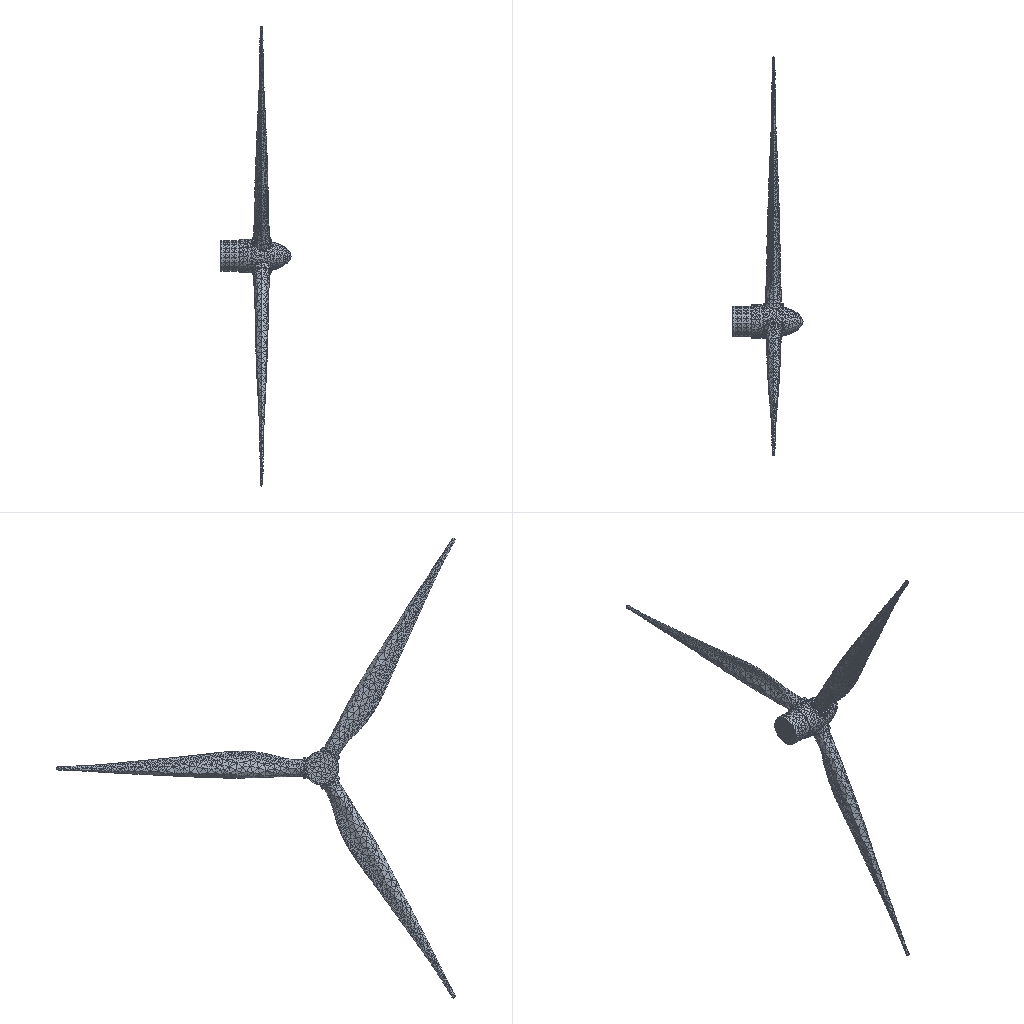Simulation study | abaqus
Set-up summary:
category,name,step,type,value,unit,region
solver,abaqus
solver,version,,,Abaqus/Standard 2020
units,not stated in the deck,,not stated
analysis,deck,,static,static
load_step,Step-1,Step-1,static
load_step,requested,,,1
mesh,nodes,,,4505
mesh,elements,,,17232
element_type,C3D4,,solid,17232
load,load commands in deck,,count,3
bc,support commands in deck,,count,5
material,MATERIAL-1,,in results
material,MATERIAL-2,,in results
check,setup vs results,,match,"per instance, exact: element labels, types and connectivity; labels of the nodes the elements use; coordinates of those nodes at SINGLE_PRECISION in 1 of 1 instance(s)"
Abaqus input file, long lists of numbers shortened:
*Heading
** Job name: Job-3 Model name: Model-load
** Generated by: Abaqus/CAE 2020
*Preprint, echo=NO, model=NO, history=NO, contact=NO
**
** PARTS
**
*Part, name=Part-1
*Node
      1,   58976.211,      121000.,   57021.883
      2,   58975.773,      121000.,   56406.227
** (4503 more lines like these left out)
*Element, type=C3D4
    1, 2870, 2871, 2872, 2873
    2, 2874, 2875, 2876, 2877
** (17230 more lines like these left out)
*Nset, nset=Set-1, generate
    1,  4505,     1
*Elset, elset=Set-1, generate
     1,  17232,      1
** Section: Section-1
*Solid Section, elset=Set-1, material=Material-1
,
*End Part
**
**
** ASSEMBLY
**
*Assembly, name=Assembly
**
*Instance, name=Part-1-1, part=Part-1
*End Instance
**
*Node
      1,   52326.004,       78000.,   56730.852
*Node
      2,   63826.004,       78000.,   56732.086
*Nset, nset=Set-1, instance=Part-1-1
   43,   44,  467,  468,  469,  470,  471,  472,  473,  474,  475,  476,  477,  478,  479,  480
  481,  482,  483,  484, 1973, 1974, 1975, 1976, 1977, 1978, 1979, 1980, 1981, 1982, 1983, 1984
** (2 more lines like these left out)
*Elset, elset=Set-1, instance=Part-1-1
  1297,  3959,  3966,  4215,  4831,  6185,  6641,  7731,  8646,  8652,  8907,  9200,  9323,  9673, 10541, 11113
 11705, 12541, 12704, 12824, 13069, 13594, 13615, 13697, 14771, 14901, 14957, 15195, 15431, 15437, 15461, 15480
** (3 more lines like these left out)
*Nset, nset=Set-2, instance=Part-1-1
   43,   44,   60,   61,  467,  468,  469,  470,  471,  472,  473,  474,  475,  476,  477,  478
  479,  480,  481,  482,  483,  484,  535,  536,  537,  538,  539,  540,  541,  542,  543,  544
** (7 more lines like these left out)
*Elset, elset=Set-2, instance=Part-1-1
  1297,  3829,  3933,  3941,  3959,  3966,  4007,  4205,  4215,  4335,  4437,  4831,  4989,  5082,  5288,  5298
  5478,  5887,  5890,  6185,  6641,  6764,  7368,  7731,  7742,  7935,  8069,  8646,  8652,  8907,  8977,  9142
** (13 more lines like these left out)
*Nset, nset=Set-3, instance=Part-1-1, generate
    1,  4505,     1
*Elset, elset=Set-3, instance=Part-1-1, generate
     1,  17232,      1
*Elset, elset=_Surf-7_S4, internal, instance=Part-1-1
   232,   317,   347,   398,  1655,  2312,  2715,  2790,  2843,  3051,  3112,  3293,  3971,  4063,  4421,  4577
  4776,  4780,  4885,  5407,  5421,  5768,  6007,  6053,  6186,  6435,  6555,  6608,  6778,  6792,  6942,  7069
** (5 more lines like these left out)
*Elset, elset=_Surf-7_S3, internal, instance=Part-1-1
   499,   574,   575,   900,  1279,  1984,  2128,  2198,  2315,  2338,  2524,  2527,  2590,  2677,  2746,  2781
  3056,  3147,  3823,  3824,  3838,  3856,  3865,  3872,  3878,  3913,  3927,  3957,  3984,  3986,  3988,  3990
** (103 more lines like these left out)
*Elset, elset=_Surf-7_S2, internal, instance=Part-1-1
    36,  2154,  2212,  2541,  3861,  3901,  3907,  4164,  4173,  4302,  4460,  4897,  5033,  5350,  5469,  5606
  5728,  5740,  5821,  5866,  6029,  6100,  6203,  6334,  6351,  6367,  6561,  6587,  6613,  6640,  6642,  6806
** (5 more lines like these left out)
*Elset, elset=_Surf-7_S1, internal, instance=Part-1-1
  3053,  3881,  4316,  4476,  5279,  5603,  5682,  6080,  6300,  6471,  6486,  6496,  6715,  7375,  7452,  7507
  7553,  8029,  8435,  8467,  8850,  9059,  9316,  9877, 10250, 10719, 11313, 11940, 12051, 12120, 12158, 12539
** (1 more lines like these left out)
*Surface, type=ELEMENT, name=Surf-7
_Surf-7_S4, S4
_Surf-7_S3, S3
_Surf-7_S2, S2
_Surf-7_S1, S1
*Elset, elset=_m_Surf-1_S3, internal, instance=Part-1-1
  4310,  9640, 14543, 14690, 14728, 14746, 14840, 14851, 14865, 14873, 14915, 15093, 15129, 15134, 15182, 15187
 15303, 15315, 15364, 15367, 15374
*Elset, elset=_m_Surf-1_S4, internal, instance=Part-1-1
  1961, 14891, 15137, 15144
*Elset, elset=_m_Surf-1_S1, internal, instance=Part-1-1
 14914, 15087, 15190, 15415
*Elset, elset=_m_Surf-1_S2, internal, instance=Part-1-1
  2071, 14906, 14910
*Surface, type=ELEMENT, name=m_Surf-1
_m_Surf-1_S3, S3
_m_Surf-1_S4, S4
_m_Surf-1_S2, S2
_m_Surf-1_S1, S1
*Elset, elset=_m_Surf-3_S3, internal, instance=Part-1-1
    54,   536,   695,   757,   994,  1039,  1801,  2267, 14907, 15018
*Elset, elset=_m_Surf-3_S4, internal, instance=Part-1-1
   195,   391,   627,   735, 13789
*Elset, elset=_m_Surf-3_S1, internal, instance=Part-1-1
   187,   218,   275,   632,   782,  1285, 15924, 16868
*Elset, elset=_m_Surf-3_S2, internal, instance=Part-1-1
   873,  1058,  1175,  1223,  1642,  1696,  2477, 14404, 15561
*Surface, type=ELEMENT, name=m_Surf-3
_m_Surf-3_S3, S3
_m_Surf-3_S4, S4
_m_Surf-3_S2, S2
_m_Surf-3_S1, S1
*Elset, elset=_m_Surf-5_S3, internal, instance=Part-1-1
  4358,  4747,  4849, 14422, 14452, 14462, 14469, 14569, 14749, 14754, 14758, 14765, 14768, 14778, 14780, 14783
 14787, 14789, 14800, 14808, 14824, 14834, 14889, 14925, 14978, 14992, 15226, 15262
*Elset, elset=_m_Surf-5_S2, internal, instance=Part-1-1
  1643,  2137, 15210
*Elset, elset=_m_Surf-5_S1, internal, instance=Part-1-1
 6768,
*Surface, type=ELEMENT, name=m_Surf-5
_m_Surf-5_S3, S3
_m_Surf-5_S2, S2
_m_Surf-5_S1, S1
*End Assembly
*Amplitude, name=Amp-1
             0.,              0.,              1.,              1.
**
** MATERIALS
**
*Material, name=Material-1
*Density
1500.,
*Elastic
 1.25e+11, 0.22
*Material, name=Material-2
*Density
7800.,
*Elastic
 2.1e+11, 0.3
** ----------------------------------------------------------------
**
** STEP: Step-1
**
*Step, name=Step-1, nlgeom=YES, inc=1000
*Static, stabilize=0.0002, allsdtol=0.05, continue=NO
0.001, 1., 1e-05, 1.
**
** BOUNDARY CONDITIONS
**
** Name: BC-1 Type: 位移/转角
*Boundary
Set-2, 1, 1
Set-2, 2, 2
Set-2, 3, 3
Set-2, 5, 5
Set-2, 6, 6
**
** LOADS
**
** Name: Load-1   Type: Gravity
*Dload
, GRAV, 9.8, 0., -1., 0.
** Name: Load-2   Type: Surface traction
*Dsload, amplitude=Amp-1
Surf-7, TRVEC, 500000., 0., 0., -1.
** Name: Load-3   Type: Rotational body force
*Dload
Set-3, CENTRIF, 0.01578,52326.,78000.,56730.9,1.,0.,0.0001071
**
** OUTPUT REQUESTS
**
*Restart, write, frequency=0
**
** FIELD OUTPUT: F-Output-1
**
*Output, field
*Node Output
CF, RF, U, UR, V
*Element Output, directions=YES
E, LE, MISES, PE, PEEQ, PEMAG, S
*Contact Output
CDISP, CSTRESS
**
** HISTORY OUTPUT: H-Output-1
**
*Output, history, variable=PRESELECT
*End Step
Results summary:
result,step,,completed,increments=19 time=1.0/1.0
result,analysis,,,static
result,last_loadstep,,,1
result,primary field,,,U
result,reaction total,,FX,47555436732.0,model units
result,reaction total,,FY,16448880401481728,model units
result,reaction total,,FZ,661485427706880.0,model units